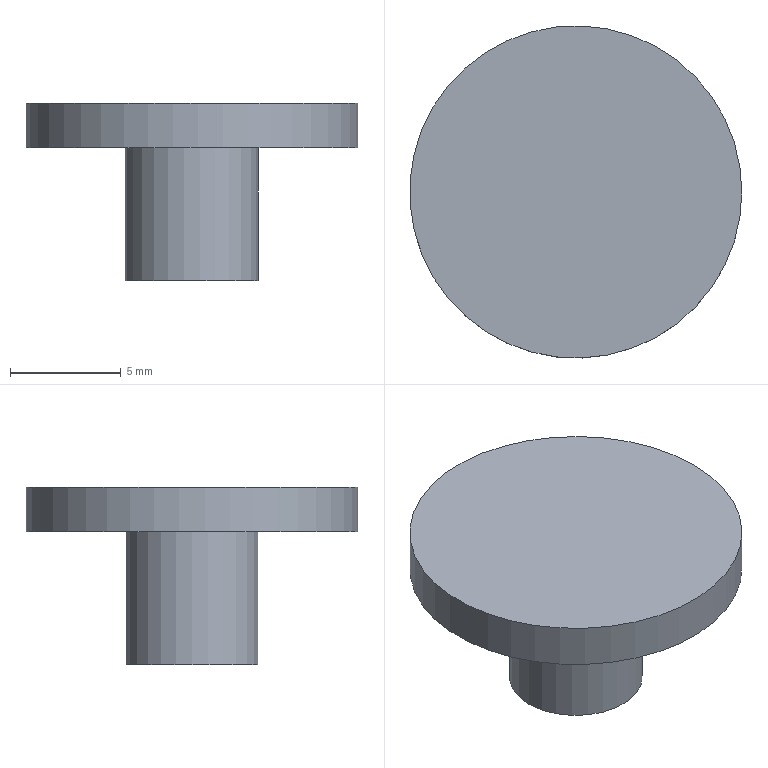Part | NX | features DATUM_CSYS 3, EXTRUDE 2, SKETCH 2, HOLE PACKAGE 1, SIMPLE HOLE 1, SYMBOLIC_THREAD 1 | 1 solid | 8 faces | box 15 x 15 x 8 mm | volume 492.132 mm3 | cylinder 3 | plane 3 | cone 2 | commonest cylinder face diameters 2.5 x1 6 x1 15 x1
STEP:
#1=CARTESIAN_POINT('',(3.,0.,6.));
#2=VERTEX_POINT('',#1);
#3=CARTESIAN_POINT('',(0.,0.,6.));
#4=DIRECTION('',(0.,0.,1.));
#5=DIRECTION('',(1.,0.,0.));
#6=AXIS2_PLACEMENT_3D('',#3,#4,#5);
#7=CIRCLE('',#6,3.);
#8=EDGE_CURVE('',#2,#2,#7,.T.);
#9=ORIENTED_EDGE('',*,*,#8,.F.);
#10=EDGE_LOOP('',(#9));
#11=FACE_BOUND('',#10,.T.);
#12=CARTESIAN_POINT('',(3.,0.,0.));
#13=VERTEX_POINT('',#12);
#14=CARTESIAN_POINT('',(0.,0.,0.));
#15=DIRECTION('',(0.,0.,1.));
#16=DIRECTION('',(1.,0.,0.));
#17=AXIS2_PLACEMENT_3D('',#14,#15,#16);
#18=CIRCLE('',#17,3.);
#19=EDGE_CURVE('',#13,#13,#18,.T.);
#20=ORIENTED_EDGE('',*,*,#19,.T.);
#21=EDGE_LOOP('',(#20));
#22=FACE_BOUND('',#21,.T.);
#23=CARTESIAN_POINT('',(0.,0.,6.));
#24=DIRECTION('',(0.,0.,-1.));
#25=DIRECTION('',(-1.,0.,0.));
#26=AXIS2_PLACEMENT_3D('',#23,#24,#25);
#27=CYLINDRICAL_SURFACE('',#26,3.);
#28=ADVANCED_FACE('',(#11,#22),#27,.T.);
#29=CARTESIAN_POINT('',(1.5,0.,0.));
#30=VERTEX_POINT('',#29);
#31=CARTESIAN_POINT('',(0.,0.,0.));
#32=DIRECTION('',(0.,0.,1.));
#33=DIRECTION('',(1.,0.,0.));
#34=AXIS2_PLACEMENT_3D('',#31,#32,#33);
#35=CIRCLE('',#34,1.5);
#36=EDGE_CURVE('',#30,#30,#35,.T.);
#37=ORIENTED_EDGE('',*,*,#36,.T.);
#38=EDGE_LOOP('',(#37));
#39=FACE_BOUND('',#38,.T.);
#40=ORIENTED_EDGE('',*,*,#19,.F.);
#41=EDGE_LOOP('',(#40));
#42=FACE_BOUND('',#41,.T.);
#43=CARTESIAN_POINT('',(0.,0.,0.));
#44=DIRECTION('',(0.,0.,1.));
#45=DIRECTION('',(1.,0.,0.));
#46=AXIS2_PLACEMENT_3D('',#43,#44,#45);
#47=PLANE('',#46);
#48=ADVANCED_FACE('',(#39,#42),#47,.F.);
#49=CARTESIAN_POINT('',(7.5,0.,8.));
#50=VERTEX_POINT('',#49);
#51=CARTESIAN_POINT('',(0.,0.,8.));
#52=DIRECTION('',(0.,0.,1.));
#53=DIRECTION('',(1.,0.,0.));
#54=AXIS2_PLACEMENT_3D('',#51,#52,#53);
#55=CIRCLE('',#54,7.5);
#56=EDGE_CURVE('',#50,#50,#55,.T.);
#57=ORIENTED_EDGE('',*,*,#56,.F.);
#58=EDGE_LOOP('',(#57));
#59=FACE_BOUND('',#58,.T.);
#60=CARTESIAN_POINT('',(7.5,0.,6.));
#61=VERTEX_POINT('',#60);
#62=CARTESIAN_POINT('',(0.,0.,6.));
#63=DIRECTION('',(0.,0.,1.));
#64=DIRECTION('',(1.,0.,0.));
#65=AXIS2_PLACEMENT_3D('',#62,#63,#64);
#66=CIRCLE('',#65,7.5);
#67=EDGE_CURVE('',#61,#61,#66,.T.);
#68=ORIENTED_EDGE('',*,*,#67,.T.);
#69=EDGE_LOOP('',(#68));
#70=FACE_BOUND('',#69,.T.);
#71=CARTESIAN_POINT('',(0.,0.,8.));
#72=DIRECTION('',(0.,0.,-1.));
#73=DIRECTION('',(-1.,0.,0.));
#74=AXIS2_PLACEMENT_3D('',#71,#72,#73);
#75=CYLINDRICAL_SURFACE('',#74,7.5);
#76=ADVANCED_FACE('',(#59,#70),#75,.T.);
#77=ORIENTED_EDGE('',*,*,#56,.T.);
#78=EDGE_LOOP('',(#77));
#79=FACE_BOUND('',#78,.T.);
#80=CARTESIAN_POINT('',(0.,0.,8.));
#81=DIRECTION('',(0.,0.,1.));
#82=DIRECTION('',(1.,0.,0.));
#83=AXIS2_PLACEMENT_3D('',#80,#81,#82);
#84=PLANE('',#83);
#85=ADVANCED_FACE('',(#79),#84,.T.);
#86=ORIENTED_EDGE('',*,*,#8,.T.);
#87=EDGE_LOOP('',(#86));
#88=FACE_BOUND('',#87,.T.);
#89=ORIENTED_EDGE('',*,*,#67,.F.);
#90=EDGE_LOOP('',(#89));
#91=FACE_BOUND('',#90,.T.);
#92=CARTESIAN_POINT('',(0.,0.,6.));
#93=DIRECTION('',(0.,0.,1.));
#94=DIRECTION('',(1.,0.,0.));
#95=AXIS2_PLACEMENT_3D('',#92,#93,#94);
#96=PLANE('',#95);
#97=ADVANCED_FACE('',(#88,#91),#96,.F.);
#98=CARTESIAN_POINT('',(1.25,0.,6.));
#99=VERTEX_POINT('',#98);
#100=CARTESIAN_POINT('',(0.,0.,6.));
#101=DIRECTION('',(0.,0.,1.));
#102=DIRECTION('',(1.,0.,0.));
#103=AXIS2_PLACEMENT_3D('',#100,#101,#102);
#104=CIRCLE('',#103,1.25);
#105=EDGE_CURVE('',#99,#99,#104,.F.);
#106=ORIENTED_EDGE('',*,*,#105,.T.);
#107=EDGE_LOOP('',(#106));
#108=FACE_BOUND('',#107,.T.);
#109=CARTESIAN_POINT('',(0.,0.,6.751));
#110=VERTEX_POINT('',#109);
#111=VERTEX_LOOP('',#110);
#112=FACE_BOUND('',#111,.T.);
#113=CARTESIAN_POINT('',(0.,0.,6.));
#114=DIRECTION('',(0.,0.,-1.));
#115=DIRECTION('',(-1.,0.,0.));
#116=AXIS2_PLACEMENT_3D('',#113,#114,#115);
#117=CONICAL_SURFACE('',#116,1.25,1.03);
#118=ADVANCED_FACE('',(#108,#112),#117,.F.);
#119=CARTESIAN_POINT('',(1.25,0.,0.25));
#120=VERTEX_POINT('',#119);
#121=CARTESIAN_POINT('',(0.,0.,0.25));
#122=DIRECTION('',(0.,0.,1.));
#123=DIRECTION('',(1.,0.,0.));
#124=AXIS2_PLACEMENT_3D('',#121,#122,#123);
#125=CIRCLE('',#124,1.25);
#126=EDGE_CURVE('',#120,#120,#125,.F.);
#127=ORIENTED_EDGE('',*,*,#126,.T.);
#128=EDGE_LOOP('',(#127));
#129=FACE_BOUND('',#128,.T.);
#130=ORIENTED_EDGE('',*,*,#105,.F.);
#131=EDGE_LOOP('',(#130));
#132=FACE_BOUND('',#131,.T.);
#133=CARTESIAN_POINT('',(0.,0.,0.));
#134=DIRECTION('',(0.,0.,1.));
#135=DIRECTION('',(1.,0.,0.));
#136=AXIS2_PLACEMENT_3D('',#133,#134,#135);
#137=CYLINDRICAL_SURFACE('',#136,1.25);
#138=ADVANCED_FACE('',(#129,#132),#137,.F.);
#139=ORIENTED_EDGE('',*,*,#126,.F.);
#140=EDGE_LOOP('',(#139));
#141=FACE_BOUND('',#140,.T.);
#142=ORIENTED_EDGE('',*,*,#36,.F.);
#143=EDGE_LOOP('',(#142));
#144=FACE_BOUND('',#143,.T.);
#145=CARTESIAN_POINT('',(0.,0.,0.));
#146=DIRECTION('',(0.,0.,-1.));
#147=DIRECTION('',(-1.,0.,0.));
#148=AXIS2_PLACEMENT_3D('',#145,#146,#147);
#149=CONICAL_SURFACE('',#148,1.5,0.7854);
#150=ADVANCED_FACE('',(#141,#144),#149,.F.);
#151=CLOSED_SHELL('',(#28,#48,#76,#85,#97,#118,#138,#150));
#152=MANIFOLD_SOLID_BREP('',#151);
#153=(LENGTH_UNIT()NAMED_UNIT(*)SI_UNIT(.MILLI.,.METRE.));
#154=UNCERTAINTY_MEASURE_WITH_UNIT(LENGTH_MEASURE(0.00001),#153,'','');
#155=(NAMED_UNIT(*)PLANE_ANGLE_UNIT()SI_UNIT($,.RADIAN.));
#156=(NAMED_UNIT(*)SI_UNIT($,.STERADIAN.)SOLID_ANGLE_UNIT());
#157=(GEOMETRIC_REPRESENTATION_CONTEXT(3)GLOBAL_UNCERTAINTY_ASSIGNED_CONTEXT((#154))GLOBAL_UNIT_ASSIGNED_CONTEXT((#153,#155,#156))REPRESENTATION_CONTEXT('',''));
#158=ADVANCED_BREP_SHAPE_REPRESENTATION('',(#152),#157);